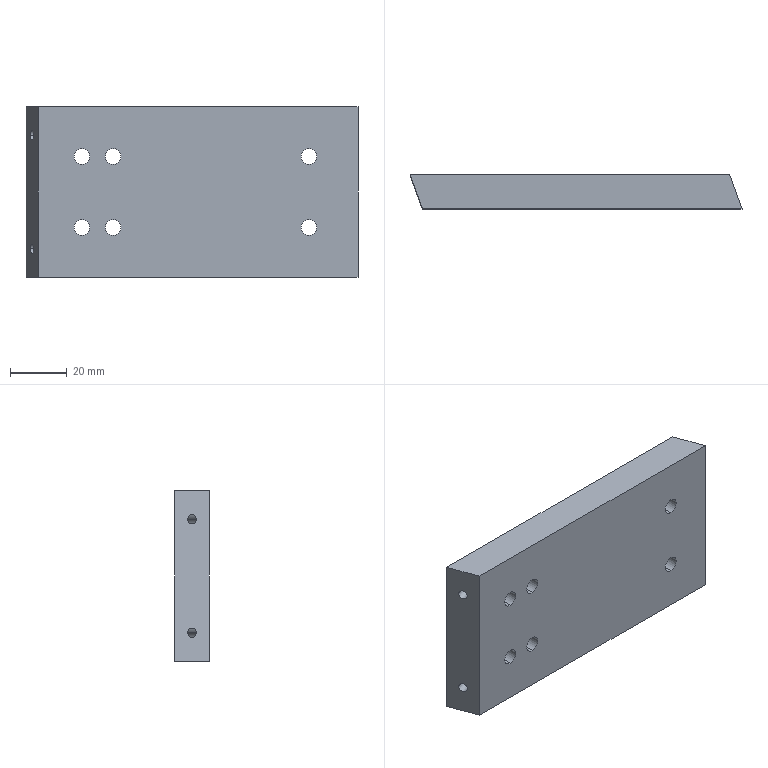Part | STEP file | vibratory feeder base plate | 1 solid | 34 faces | box 116.996 x 12 x 60 mm | volume 79045 mm3 | cylinder 20 | cone 8 | plane 6 | commonest cylinder face diameters 5.5 x12 3.3 x8